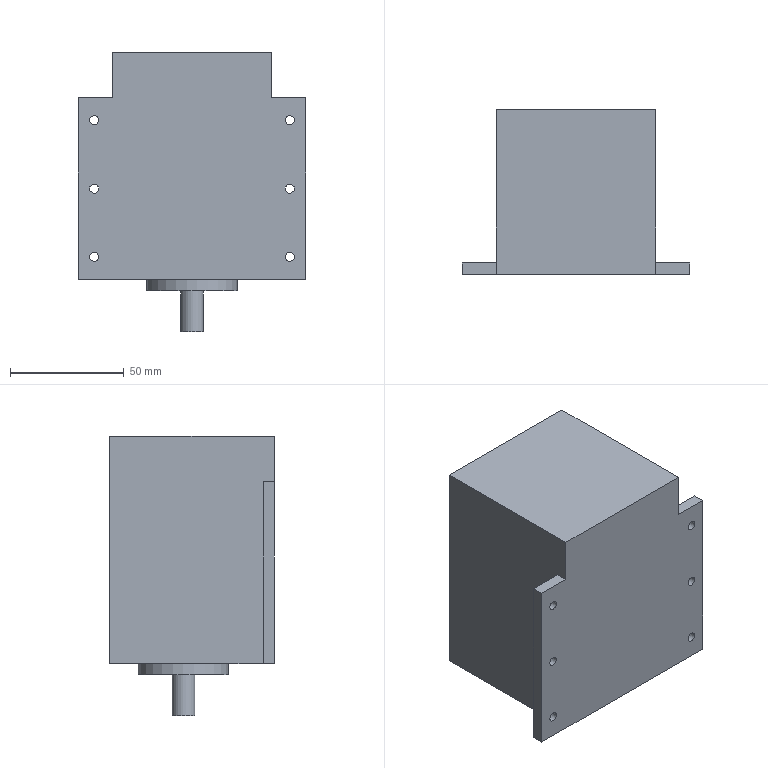Part | STEP file | tieqiandianji | 1 solid | 22 faces | box 100 x 72.5 x 123 mm | volume 526820 mm3 | plane 14 | cylinder 8 | commonest cylinder face diameters 4 x6 10 x1 40 x1